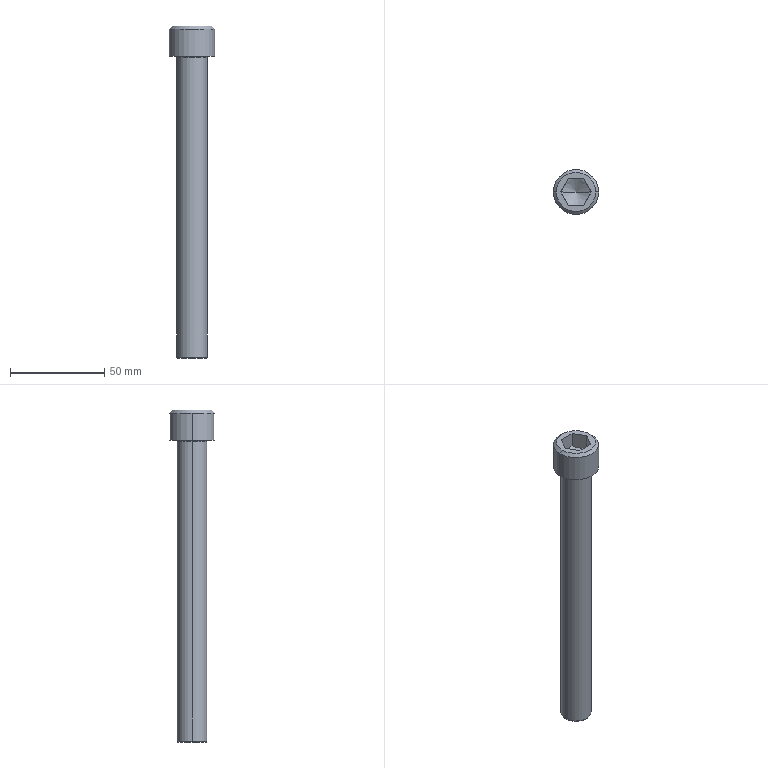Part | Creo | 1 solid | 23 faces | box 24 x 24 x 176 mm | volume 37645 mm3 | plane 9 | cone 6 | cylinder 4 | torus 4 | commonest cylinder face diameters 16 x2 24 x2
STEP:
#1=CARTESIAN_POINT('',(0.,0.,0.));
#2=DIRECTION('',(0.,0.,1.));
#3=DIRECTION('',(1.,0.,0.));
#4=AXIS2_PLACEMENT_3D('',#1,#2,#3);
#5=CARTESIAN_POINT('',(-11.917,-115.,300.5));
#6=VERTEX_POINT('',#5);
#7=CARTESIAN_POINT('',(-15.959,-108.,300.5));
#8=VERTEX_POINT('',#7);
#9=CARTESIAN_POINT('',(-11.917,-115.,300.5));
#10=CARTESIAN_POINT('',(-12.137,-114.619,300.373));
#11=CARTESIAN_POINT('',(-12.578,-113.855,300.149));
#12=CARTESIAN_POINT('',(-13.254,-112.685,299.927));
#13=CARTESIAN_POINT('',(-13.936,-111.504,299.849));
#14=CARTESIAN_POINT('',(-14.621,-110.317,299.927));
#15=CARTESIAN_POINT('',(-15.295,-109.15,300.148));
#16=CARTESIAN_POINT('',(-15.738,-108.382,300.373));
#17=CARTESIAN_POINT('',(-15.959,-108.,300.5));
#18=B_SPLINE_CURVE_WITH_KNOTS('',3,(#9,#10,#11,#12,#13,#14,#15,#16,#17),.UNSPECIFIED.,.F.,.F.,(4,1,1,1,1,1,4),(0.,0.1667,0.3333,0.5,0.6667,0.8333,1.),.UNSPECIFIED.);
#19=EDGE_CURVE('',#6,#8,#18,.T.);
#20=ORIENTED_EDGE('',*,*,#19,.F.);
#21=CARTESIAN_POINT('',(-20.,-115.,295.833));
#22=VERTEX_POINT('',#21);
#23=CARTESIAN_POINT('',(-20.,-115.,295.833));
#24=DIRECTION('',(0.866,0.,0.5));
#25=VECTOR('',#24,9.333);
#26=LINE('',#23,#25);
#27=EDGE_CURVE('',#22,#6,#26,.T.);
#28=ORIENTED_EDGE('',*,*,#27,.F.);
#29=CARTESIAN_POINT('',(-28.083,-115.,300.5));
#30=VERTEX_POINT('',#29);
#31=CARTESIAN_POINT('',(-20.,-115.,295.833));
#32=DIRECTION('',(-0.866,0.,0.5));
#33=VECTOR('',#32,9.333);
#34=LINE('',#31,#33);
#35=EDGE_CURVE('',#22,#30,#34,.T.);
#36=ORIENTED_EDGE('',*,*,#35,.T.);
#37=CARTESIAN_POINT('',(-24.041,-108.,300.5));
#38=VERTEX_POINT('',#37);
#39=CARTESIAN_POINT('',(-24.041,-108.,300.5));
#40=CARTESIAN_POINT('',(-24.261,-108.381,300.373));
#41=CARTESIAN_POINT('',(-24.703,-109.145,300.149));
#42=CARTESIAN_POINT('',(-25.378,-110.315,299.927));
#43=CARTESIAN_POINT('',(-26.06,-111.496,299.849));
#44=CARTESIAN_POINT('',(-26.745,-112.683,299.927));
#45=CARTESIAN_POINT('',(-27.419,-113.85,300.148));
#46=CARTESIAN_POINT('',(-27.862,-114.618,300.373));
#47=CARTESIAN_POINT('',(-28.083,-115.,300.5));
#48=B_SPLINE_CURVE_WITH_KNOTS('',3,(#39,#40,#41,#42,#43,#44,#45,#46,#47),.UNSPECIFIED.,.F.,.F.,(4,1,1,1,1,1,4),(0.,0.1667,0.3333,0.5,0.6667,0.8333,1.),.UNSPECIFIED.);
#49=EDGE_CURVE('',#38,#30,#48,.T.);
#50=ORIENTED_EDGE('',*,*,#49,.F.);
#51=CARTESIAN_POINT('',(-15.959,-108.,300.5));
#52=CARTESIAN_POINT('',(-16.396,-108.,300.374));
#53=CARTESIAN_POINT('',(-17.277,-108.,300.15));
#54=CARTESIAN_POINT('',(-18.631,-108.,299.927));
#55=CARTESIAN_POINT('',(-19.998,-108.,299.849));
#56=CARTESIAN_POINT('',(-21.363,-108.,299.926));
#57=CARTESIAN_POINT('',(-22.717,-108.,300.149));
#58=CARTESIAN_POINT('',(-23.601,-108.,300.373));
#59=CARTESIAN_POINT('',(-24.041,-108.,300.5));
#60=B_SPLINE_CURVE_WITH_KNOTS('',3,(#51,#52,#53,#54,#55,#56,#57,#58,#59),.UNSPECIFIED.,.F.,.F.,(4,1,1,1,1,1,4),(0.,0.1667,0.3333,0.5,0.6667,0.8333,1.),.UNSPECIFIED.);
#61=EDGE_CURVE('',#8,#38,#60,.T.);
#62=ORIENTED_EDGE('',*,*,#61,.F.);
#63=EDGE_LOOP('',(#20,#28,#36,#50,#62));
#64=FACE_OUTER_BOUND('',#63,.F.);
#65=CARTESIAN_POINT('',(-20.,-115.,298.22));
#66=DIRECTION('',(0.,0.,1.));
#67=DIRECTION('',(1.,0.,0.));
#68=AXIS2_PLACEMENT_3D('',#65,#66,#67);
#69=CONICAL_SURFACE('',#68,4.135,60.);
#70=ADVANCED_FACE('',(#64),#69,.F.);
#71=CARTESIAN_POINT('',(-15.959,-108.,308.5));
#72=VERTEX_POINT('',#71);
#73=CARTESIAN_POINT('',(-11.917,-115.,308.5));
#74=VERTEX_POINT('',#73);
#75=CARTESIAN_POINT('',(-15.959,-108.,308.5));
#76=DIRECTION('',(0.5,-0.866,0.));
#77=VECTOR('',#76,8.083);
#78=LINE('',#75,#77);
#79=EDGE_CURVE('',#72,#74,#78,.T.);
#80=ORIENTED_EDGE('',*,*,#79,.T.);
#81=CARTESIAN_POINT('',(-11.917,-115.,308.5));
#82=DIRECTION('',(0.,0.,-1.));
#83=VECTOR('',#82,8.);
#84=LINE('',#81,#83);
#85=EDGE_CURVE('',#74,#6,#84,.T.);
#86=ORIENTED_EDGE('',*,*,#85,.T.);
#87=ORIENTED_EDGE('',*,*,#19,.T.);
#88=CARTESIAN_POINT('',(-15.959,-108.,308.5));
#89=DIRECTION('',(0.,0.,-1.));
#90=VECTOR('',#89,8.);
#91=LINE('',#88,#90);
#92=EDGE_CURVE('',#72,#8,#91,.T.);
#93=ORIENTED_EDGE('',*,*,#92,.F.);
#94=EDGE_LOOP('',(#80,#86,#87,#93));
#95=FACE_OUTER_BOUND('',#94,.F.);
#96=CARTESIAN_POINT('',(-15.959,-108.,300.5));
#97=DIRECTION('',(-0.866,-0.5,0.));
#98=DIRECTION('',(0.5,-0.866,0.));
#99=AXIS2_PLACEMENT_3D('',#96,#97,#98);
#100=PLANE('',#99);
#101=ADVANCED_FACE('',(#95),#100,.T.);
#102=CARTESIAN_POINT('',(-9.6,-115.,308.5));
#103=VERTEX_POINT('',#102);
#104=CARTESIAN_POINT('',(-30.4,-115.,308.5));
#105=VERTEX_POINT('',#104);
#106=CARTESIAN_POINT('',(-20.,-115.,308.5));
#107=DIRECTION('',(0.,0.,1.));
#108=DIRECTION('',(1.,0.,0.));
#109=AXIS2_PLACEMENT_3D('',#106,#107,#108);
#110=CIRCLE('',#109,10.4);
#111=EDGE_CURVE('',#103,#105,#110,.T.);
#112=ORIENTED_EDGE('',*,*,#111,.F.);
#113=CARTESIAN_POINT('',(-20.,-115.,308.5));
#114=DIRECTION('',(0.,0.,1.));
#115=DIRECTION('',(-1.,0.,0.));
#116=AXIS2_PLACEMENT_3D('',#113,#114,#115);
#117=CIRCLE('',#116,10.4);
#118=EDGE_CURVE('',#105,#103,#117,.T.);
#119=ORIENTED_EDGE('',*,*,#118,.F.);
#120=EDGE_LOOP('',(#112,#119));
#121=FACE_OUTER_BOUND('',#120,.F.);
#122=CARTESIAN_POINT('',(-15.959,-122.,308.5));
#123=VERTEX_POINT('',#122);
#124=CARTESIAN_POINT('',(-11.917,-115.,308.5));
#125=DIRECTION('',(-0.5,-0.866,0.));
#126=VECTOR('',#125,8.083);
#127=LINE('',#124,#126);
#128=EDGE_CURVE('',#74,#123,#127,.T.);
#129=ORIENTED_EDGE('',*,*,#128,.F.);
#130=ORIENTED_EDGE('',*,*,#79,.F.);
#131=CARTESIAN_POINT('',(-24.041,-108.,308.5));
#132=VERTEX_POINT('',#131);
#133=CARTESIAN_POINT('',(-15.959,-108.,308.5));
#134=DIRECTION('',(-1.,0.,0.));
#135=VECTOR('',#134,8.083);
#136=LINE('',#133,#135);
#137=EDGE_CURVE('',#72,#132,#136,.T.);
#138=ORIENTED_EDGE('',*,*,#137,.T.);
#139=CARTESIAN_POINT('',(-28.083,-115.,308.5));
#140=VERTEX_POINT('',#139);
#141=CARTESIAN_POINT('',(-28.083,-115.,308.5));
#142=DIRECTION('',(0.5,0.866,0.));
#143=VECTOR('',#142,8.083);
#144=LINE('',#141,#143);
#145=EDGE_CURVE('',#140,#132,#144,.T.);
#146=ORIENTED_EDGE('',*,*,#145,.F.);
#147=CARTESIAN_POINT('',(-24.041,-122.,308.5));
#148=VERTEX_POINT('',#147);
#149=CARTESIAN_POINT('',(-24.041,-122.,308.5));
#150=DIRECTION('',(-0.5,0.866,0.));
#151=VECTOR('',#150,8.083);
#152=LINE('',#149,#151);
#153=EDGE_CURVE('',#148,#140,#152,.T.);
#154=ORIENTED_EDGE('',*,*,#153,.F.);
#155=CARTESIAN_POINT('',(-24.041,-122.,308.5));
#156=DIRECTION('',(1.,0.,0.));
#157=VECTOR('',#156,8.083);
#158=LINE('',#155,#157);
#159=EDGE_CURVE('',#148,#123,#158,.T.);
#160=ORIENTED_EDGE('',*,*,#159,.T.);
#161=EDGE_LOOP('',(#129,#130,#138,#146,#154,#160));
#162=FACE_BOUND('',#161,.F.);
#163=CARTESIAN_POINT('',(-20.,-115.,308.5));
#164=DIRECTION('',(0.,0.,1.));
#165=DIRECTION('',(1.,0.,0.));
#166=AXIS2_PLACEMENT_3D('',#163,#164,#165);
#167=PLANE('',#166);
#168=ADVANCED_FACE('',(#121,#162),#167,.T.);
#169=CARTESIAN_POINT('',(-8.,-115.,306.9));
#170=VERTEX_POINT('',#169);
#171=CARTESIAN_POINT('',(-32.,-115.,306.9));
#172=VERTEX_POINT('',#171);
#173=CARTESIAN_POINT('',(-20.,-115.,306.9));
#174=DIRECTION('',(0.,0.,1.));
#175=DIRECTION('',(1.,0.,0.));
#176=AXIS2_PLACEMENT_3D('',#173,#174,#175);
#177=CIRCLE('',#176,12.);
#178=EDGE_CURVE('',#170,#172,#177,.T.);
#179=ORIENTED_EDGE('',*,*,#178,.F.);
#180=CARTESIAN_POINT('',(-9.6,-115.,308.5));
#181=DIRECTION('',(0.7071,0.,-0.7071));
#182=VECTOR('',#181,2.263);
#183=LINE('',#180,#182);
#184=EDGE_CURVE('',#103,#170,#183,.T.);
#185=ORIENTED_EDGE('',*,*,#184,.F.);
#186=ORIENTED_EDGE('',*,*,#111,.T.);
#187=CARTESIAN_POINT('',(-30.4,-115.,308.5));
#188=DIRECTION('',(-0.7071,0.,-0.7071));
#189=VECTOR('',#188,2.263);
#190=LINE('',#187,#189);
#191=EDGE_CURVE('',#105,#172,#190,.T.);
#192=ORIENTED_EDGE('',*,*,#191,.T.);
#193=EDGE_LOOP('',(#179,#185,#186,#192));
#194=FACE_OUTER_BOUND('',#193,.F.);
#195=CARTESIAN_POINT('',(-20.,-115.,307.7));
#196=DIRECTION('',(0.,0.,-1.));
#197=DIRECTION('',(-1.,0.,0.));
#198=AXIS2_PLACEMENT_3D('',#195,#196,#197);
#199=CONICAL_SURFACE('',#198,11.2,45.);
#200=ADVANCED_FACE('',(#194),#199,.T.);
#201=ORIENTED_EDGE('',*,*,#178,.T.);
#202=CARTESIAN_POINT('',(-32.,-115.,292.5));
#203=VERTEX_POINT('',#202);
#204=CARTESIAN_POINT('',(-32.,-115.,292.5));
#205=DIRECTION('',(0.,0.,1.));
#206=VECTOR('',#205,14.4);
#207=LINE('',#204,#206);
#208=EDGE_CURVE('',#203,#172,#207,.T.);
#209=ORIENTED_EDGE('',*,*,#208,.F.);
#210=CARTESIAN_POINT('',(-8.,-115.,292.5));
#211=VERTEX_POINT('',#210);
#212=CARTESIAN_POINT('',(-20.,-115.,292.5));
#213=DIRECTION('',(0.,0.,-1.));
#214=DIRECTION('',(-1.,0.,0.));
#215=AXIS2_PLACEMENT_3D('',#212,#213,#214);
#216=CIRCLE('',#215,12.);
#217=EDGE_CURVE('',#203,#211,#216,.T.);
#218=ORIENTED_EDGE('',*,*,#217,.T.);
#219=CARTESIAN_POINT('',(-8.,-115.,292.5));
#220=DIRECTION('',(0.,0.,1.));
#221=VECTOR('',#220,14.4);
#222=LINE('',#219,#221);
#223=EDGE_CURVE('',#211,#170,#222,.T.);
#224=ORIENTED_EDGE('',*,*,#223,.T.);
#225=EDGE_LOOP('',(#201,#209,#218,#224));
#226=FACE_OUTER_BOUND('',#225,.F.);
#227=CARTESIAN_POINT('',(-20.,-115.,292.5));
#228=DIRECTION('',(0.,0.,1.));
#229=DIRECTION('',(1.,0.,0.));
#230=AXIS2_PLACEMENT_3D('',#227,#228,#229);
#231=CYLINDRICAL_SURFACE('',#230,12.);
#232=ADVANCED_FACE('',(#226),#231,.T.);
#233=CARTESIAN_POINT('',(-20.,-115.,306.9));
#234=DIRECTION('',(0.,0.,1.));
#235=DIRECTION('',(-1.,0.,0.));
#236=AXIS2_PLACEMENT_3D('',#233,#234,#235);
#237=CIRCLE('',#236,12.);
#238=EDGE_CURVE('',#172,#170,#237,.T.);
#239=ORIENTED_EDGE('',*,*,#238,.T.);
#240=ORIENTED_EDGE('',*,*,#223,.F.);
#241=CARTESIAN_POINT('',(-20.,-115.,292.5));
#242=DIRECTION('',(0.,0.,-1.));
#243=DIRECTION('',(1.,0.,0.));
#244=AXIS2_PLACEMENT_3D('',#241,#242,#243);
#245=CIRCLE('',#244,12.);
#246=EDGE_CURVE('',#211,#203,#245,.T.);
#247=ORIENTED_EDGE('',*,*,#246,.T.);
#248=ORIENTED_EDGE('',*,*,#208,.T.);
#249=EDGE_LOOP('',(#239,#240,#247,#248));
#250=FACE_OUTER_BOUND('',#249,.F.);
#251=CARTESIAN_POINT('',(-20.,-115.,292.5));
#252=DIRECTION('',(0.,0.,1.));
#253=DIRECTION('',(1.,0.,0.));
#254=AXIS2_PLACEMENT_3D('',#251,#252,#253);
#255=CYLINDRICAL_SURFACE('',#254,12.);
#256=ADVANCED_FACE('',(#250),#255,.T.);
#257=ORIENTED_EDGE('',*,*,#238,.F.);
#258=ORIENTED_EDGE('',*,*,#191,.F.);
#259=ORIENTED_EDGE('',*,*,#118,.T.);
#260=ORIENTED_EDGE('',*,*,#184,.T.);
#261=EDGE_LOOP('',(#257,#258,#259,#260));
#262=FACE_OUTER_BOUND('',#261,.F.);
#263=CARTESIAN_POINT('',(-20.,-115.,307.7));
#264=DIRECTION('',(0.,0.,-1.));
#265=DIRECTION('',(-1.,0.,0.));
#266=AXIS2_PLACEMENT_3D('',#263,#264,#265);
#267=CONICAL_SURFACE('',#266,11.2,45.);
#268=ADVANCED_FACE('',(#262),#267,.T.);
#269=ORIENTED_EDGE('',*,*,#246,.F.);
#270=ORIENTED_EDGE('',*,*,#217,.F.);
#271=EDGE_LOOP('',(#269,#270));
#272=FACE_OUTER_BOUND('',#271,.F.);
#273=CARTESIAN_POINT('',(-11.4,-115.,292.5));
#274=VERTEX_POINT('',#273);
#275=CARTESIAN_POINT('',(-28.6,-115.,292.5));
#276=VERTEX_POINT('',#275);
#277=CARTESIAN_POINT('',(-20.,-115.,292.5));
#278=DIRECTION('',(0.,0.,1.));
#279=DIRECTION('',(1.,0.,0.));
#280=AXIS2_PLACEMENT_3D('',#277,#278,#279);
#281=CIRCLE('',#280,8.6);
#282=EDGE_CURVE('',#274,#276,#281,.T.);
#283=ORIENTED_EDGE('',*,*,#282,.F.);
#284=CARTESIAN_POINT('',(-20.,-115.,292.5));
#285=DIRECTION('',(0.,0.,1.));
#286=DIRECTION('',(-1.,0.,0.));
#287=AXIS2_PLACEMENT_3D('',#284,#285,#286);
#288=CIRCLE('',#287,8.6);
#289=EDGE_CURVE('',#276,#274,#288,.T.);
#290=ORIENTED_EDGE('',*,*,#289,.F.);
#291=EDGE_LOOP('',(#283,#290));
#292=FACE_BOUND('',#291,.F.);
#293=CARTESIAN_POINT('',(-20.,-115.,292.5));
#294=DIRECTION('',(0.,0.,1.));
#295=DIRECTION('',(1.,0.,0.));
#296=AXIS2_PLACEMENT_3D('',#293,#294,#295);
#297=PLANE('',#296);
#298=ADVANCED_FACE('',(#272,#292),#297,.F.);
#299=ORIENTED_EDGE('',*,*,#282,.T.);
#300=CARTESIAN_POINT('',(-28.176,-115.,292.324));
#301=VERTEX_POINT('',#300);
#302=CARTESIAN_POINT('',(-28.6,-115.,291.9));
#303=DIRECTION('',(0.,1.,0.));
#304=DIRECTION('',(0.,0.,1.));
#305=AXIS2_PLACEMENT_3D('',#302,#303,#304);
#306=CIRCLE('',#305,0.6);
#307=EDGE_CURVE('',#276,#301,#306,.T.);
#308=ORIENTED_EDGE('',*,*,#307,.T.);
#309=CARTESIAN_POINT('',(-11.824,-115.,292.324));
#310=VERTEX_POINT('',#309);
#311=CARTESIAN_POINT('',(-20.,-115.,292.324));
#312=DIRECTION('',(0.,0.,1.));
#313=DIRECTION('',(1.,0.,0.));
#314=AXIS2_PLACEMENT_3D('',#311,#312,#313);
#315=CIRCLE('',#314,8.176);
#316=EDGE_CURVE('',#310,#301,#315,.T.);
#317=ORIENTED_EDGE('',*,*,#316,.F.);
#318=CARTESIAN_POINT('',(-11.4,-115.,291.9));
#319=DIRECTION('',(0.,-1.,0.));
#320=DIRECTION('',(0.,0.,1.));
#321=AXIS2_PLACEMENT_3D('',#318,#319,#320);
#322=CIRCLE('',#321,0.6);
#323=EDGE_CURVE('',#274,#310,#322,.T.);
#324=ORIENTED_EDGE('',*,*,#323,.F.);
#325=EDGE_LOOP('',(#299,#308,#317,#324));
#326=FACE_OUTER_BOUND('',#325,.F.);
#327=CARTESIAN_POINT('',(-20.,-115.,291.9));
#328=DIRECTION('',(0.,0.,1.));
#329=DIRECTION('',(1.,0.,0.));
#330=AXIS2_PLACEMENT_3D('',#327,#328,#329);
#331=TOROIDAL_SURFACE('',#330,8.6,0.6);
#332=ADVANCED_FACE('',(#326),#331,.F.);
#333=ORIENTED_EDGE('',*,*,#289,.T.);
#334=ORIENTED_EDGE('',*,*,#323,.T.);
#335=CARTESIAN_POINT('',(-20.,-115.,292.324));
#336=DIRECTION('',(0.,0.,1.));
#337=DIRECTION('',(-1.,0.,0.));
#338=AXIS2_PLACEMENT_3D('',#335,#336,#337);
#339=CIRCLE('',#338,8.176);
#340=EDGE_CURVE('',#301,#310,#339,.T.);
#341=ORIENTED_EDGE('',*,*,#340,.F.);
#342=ORIENTED_EDGE('',*,*,#307,.F.);
#343=EDGE_LOOP('',(#333,#334,#341,#342));
#344=FACE_OUTER_BOUND('',#343,.F.);
#345=CARTESIAN_POINT('',(-20.,-115.,291.9));
#346=DIRECTION('',(0.,0.,1.));
#347=DIRECTION('',(1.,0.,0.));
#348=AXIS2_PLACEMENT_3D('',#345,#346,#347);
#349=TOROIDAL_SURFACE('',#348,8.6,0.6);
#350=ADVANCED_FACE('',(#344),#349,.F.);
#351=CARTESIAN_POINT('',(-28.,-115.,291.9));
#352=VERTEX_POINT('',#351);
#353=CARTESIAN_POINT('',(-12.,-115.,291.9));
#354=VERTEX_POINT('',#353);
#355=CARTESIAN_POINT('',(-20.,-115.,291.9));
#356=DIRECTION('',(0.,0.,1.));
#357=DIRECTION('',(-1.,0.,0.));
#358=AXIS2_PLACEMENT_3D('',#355,#356,#357);
#359=CIRCLE('',#358,8.);
#360=EDGE_CURVE('',#352,#354,#359,.T.);
#361=ORIENTED_EDGE('',*,*,#360,.F.);
#362=CARTESIAN_POINT('',(-28.6,-115.,291.9));
#363=DIRECTION('',(0.,1.,0.));
#364=DIRECTION('',(0.7071,0.,0.7071));
#365=AXIS2_PLACEMENT_3D('',#362,#363,#364);
#366=CIRCLE('',#365,0.6);
#367=EDGE_CURVE('',#301,#352,#366,.T.);
#368=ORIENTED_EDGE('',*,*,#367,.F.);
#369=ORIENTED_EDGE('',*,*,#340,.T.);
#370=CARTESIAN_POINT('',(-11.4,-115.,291.9));
#371=DIRECTION('',(0.,-1.,0.));
#372=DIRECTION('',(-0.7071,0.,0.7071));
#373=AXIS2_PLACEMENT_3D('',#370,#371,#372);
#374=CIRCLE('',#373,0.6);
#375=EDGE_CURVE('',#310,#354,#374,.T.);
#376=ORIENTED_EDGE('',*,*,#375,.T.);
#377=EDGE_LOOP('',(#361,#368,#369,#376));
#378=FACE_OUTER_BOUND('',#377,.F.);
#379=CARTESIAN_POINT('',(-20.,-115.,291.9));
#380=DIRECTION('',(0.,0.,1.));
#381=DIRECTION('',(1.,0.,0.));
#382=AXIS2_PLACEMENT_3D('',#379,#380,#381);
#383=TOROIDAL_SURFACE('',#382,8.6,0.6);
#384=ADVANCED_FACE('',(#378),#383,.F.);
#385=CARTESIAN_POINT('',(-12.,-115.,133.));
#386=VERTEX_POINT('',#385);
#387=CARTESIAN_POINT('',(-28.,-115.,133.));
#388=VERTEX_POINT('',#387);
#389=CARTESIAN_POINT('',(-20.,-115.,133.));
#390=DIRECTION('',(0.,0.,-1.));
#391=DIRECTION('',(1.,0.,0.));
#392=AXIS2_PLACEMENT_3D('',#389,#390,#391);
#393=CIRCLE('',#392,8.);
#394=EDGE_CURVE('',#386,#388,#393,.T.);
#395=ORIENTED_EDGE('',*,*,#394,.T.);
#396=CARTESIAN_POINT('',(-28.,-115.,133.));
#397=DIRECTION('',(0.,0.,1.));
#398=VECTOR('',#397,158.9);
#399=LINE('',#396,#398);
#400=EDGE_CURVE('',#388,#352,#399,.T.);
#401=ORIENTED_EDGE('',*,*,#400,.T.);
#402=ORIENTED_EDGE('',*,*,#360,.T.);
#403=CARTESIAN_POINT('',(-12.,-115.,133.));
#404=DIRECTION('',(0.,0.,1.));
#405=VECTOR('',#404,158.9);
#406=LINE('',#403,#405);
#407=EDGE_CURVE('',#386,#354,#406,.T.);
#408=ORIENTED_EDGE('',*,*,#407,.F.);
#409=EDGE_LOOP('',(#395,#401,#402,#408));
#410=FACE_OUTER_BOUND('',#409,.F.);
#411=CARTESIAN_POINT('',(-20.,-115.,132.5));
#412=DIRECTION('',(0.,0.,1.));
#413=DIRECTION('',(1.,0.,0.));
#414=AXIS2_PLACEMENT_3D('',#411,#412,#413);
#415=CYLINDRICAL_SURFACE('',#414,8.);
#416=ADVANCED_FACE('',(#410),#415,.T.);
#417=CARTESIAN_POINT('',(-12.5,-115.,132.5));
#418=VERTEX_POINT('',#417);
#419=CARTESIAN_POINT('',(-27.5,-115.,132.5));
#420=VERTEX_POINT('',#419);
#421=CARTESIAN_POINT('',(-20.,-115.,132.5));
#422=DIRECTION('',(0.,0.,-1.));
#423=DIRECTION('',(1.,0.,0.));
#424=AXIS2_PLACEMENT_3D('',#421,#422,#423);
#425=CIRCLE('',#424,7.5);
#426=EDGE_CURVE('',#418,#420,#425,.T.);
#427=ORIENTED_EDGE('',*,*,#426,.T.);
#428=CARTESIAN_POINT('',(-27.5,-115.,132.5));
#429=DIRECTION('',(-0.7071,0.,0.7071));
#430=VECTOR('',#429,0.7071);
#431=LINE('',#428,#430);
#432=EDGE_CURVE('',#420,#388,#431,.T.);
#433=ORIENTED_EDGE('',*,*,#432,.T.);
#434=ORIENTED_EDGE('',*,*,#394,.F.);
#435=CARTESIAN_POINT('',(-12.5,-115.,132.5));
#436=DIRECTION('',(0.7071,0.,0.7071));
#437=VECTOR('',#436,0.7071);
#438=LINE('',#435,#437);
#439=EDGE_CURVE('',#418,#386,#438,.T.);
#440=ORIENTED_EDGE('',*,*,#439,.F.);
#441=EDGE_LOOP('',(#427,#433,#434,#440));
#442=FACE_OUTER_BOUND('',#441,.F.);
#443=CARTESIAN_POINT('',(-20.,-115.,132.75));
#444=DIRECTION('',(0.,0.,1.));
#445=DIRECTION('',(1.,0.,0.));
#446=AXIS2_PLACEMENT_3D('',#443,#444,#445);
#447=CONICAL_SURFACE('',#446,7.75,45.);
#448=ADVANCED_FACE('',(#442),#447,.T.);
#449=ORIENTED_EDGE('',*,*,#426,.F.);
#450=CARTESIAN_POINT('',(-20.,-115.,132.5));
#451=DIRECTION('',(0.,0.,-1.));
#452=DIRECTION('',(-1.,0.,0.));
#453=AXIS2_PLACEMENT_3D('',#450,#451,#452);
#454=CIRCLE('',#453,7.5);
#455=EDGE_CURVE('',#420,#418,#454,.T.);
#456=ORIENTED_EDGE('',*,*,#455,.F.);
#457=EDGE_LOOP('',(#449,#456));
#458=FACE_OUTER_BOUND('',#457,.F.);
#459=CARTESIAN_POINT('',(-20.,-115.,132.5));
#460=DIRECTION('',(0.,0.,1.));
#461=DIRECTION('',(1.,0.,0.));
#462=AXIS2_PLACEMENT_3D('',#459,#460,#461);
#463=PLANE('',#462);
#464=ADVANCED_FACE('',(#458),#463,.F.);
#465=ORIENTED_EDGE('',*,*,#455,.T.);
#466=ORIENTED_EDGE('',*,*,#439,.T.);
#467=CARTESIAN_POINT('',(-20.,-115.,133.));
#468=DIRECTION('',(0.,0.,-1.));
#469=DIRECTION('',(-1.,0.,0.));
#470=AXIS2_PLACEMENT_3D('',#467,#468,#469);
#471=CIRCLE('',#470,8.);
#472=EDGE_CURVE('',#388,#386,#471,.T.);
#473=ORIENTED_EDGE('',*,*,#472,.F.);
#474=ORIENTED_EDGE('',*,*,#432,.F.);
#475=EDGE_LOOP('',(#465,#466,#473,#474));
#476=FACE_OUTER_BOUND('',#475,.F.);
#477=CARTESIAN_POINT('',(-20.,-115.,132.75));
#478=DIRECTION('',(0.,0.,1.));
#479=DIRECTION('',(1.,0.,0.));
#480=AXIS2_PLACEMENT_3D('',#477,#478,#479);
#481=CONICAL_SURFACE('',#480,7.75,45.);
#482=ADVANCED_FACE('',(#476),#481,.T.);
#483=ORIENTED_EDGE('',*,*,#472,.T.);
#484=ORIENTED_EDGE('',*,*,#407,.T.);
#485=CARTESIAN_POINT('',(-20.,-115.,291.9));
#486=DIRECTION('',(0.,0.,1.));
#487=DIRECTION('',(1.,0.,0.));
#488=AXIS2_PLACEMENT_3D('',#485,#486,#487);
#489=CIRCLE('',#488,8.);
#490=EDGE_CURVE('',#354,#352,#489,.T.);
#491=ORIENTED_EDGE('',*,*,#490,.T.);
#492=ORIENTED_EDGE('',*,*,#400,.F.);
#493=EDGE_LOOP('',(#483,#484,#491,#492));
#494=FACE_OUTER_BOUND('',#493,.F.);
#495=CARTESIAN_POINT('',(-20.,-115.,132.5));
#496=DIRECTION('',(0.,0.,1.));
#497=DIRECTION('',(1.,0.,0.));
#498=AXIS2_PLACEMENT_3D('',#495,#496,#497);
#499=CYLINDRICAL_SURFACE('',#498,8.);
#500=ADVANCED_FACE('',(#494),#499,.T.);
#501=ORIENTED_EDGE('',*,*,#490,.F.);
#502=ORIENTED_EDGE('',*,*,#375,.F.);
#503=ORIENTED_EDGE('',*,*,#316,.T.);
#504=ORIENTED_EDGE('',*,*,#367,.T.);
#505=EDGE_LOOP('',(#501,#502,#503,#504));
#506=FACE_OUTER_BOUND('',#505,.F.);
#507=CARTESIAN_POINT('',(-20.,-115.,291.9));
#508=DIRECTION('',(0.,0.,1.));
#509=DIRECTION('',(1.,0.,0.));
#510=AXIS2_PLACEMENT_3D('',#507,#508,#509);
#511=TOROIDAL_SURFACE('',#510,8.6,0.6);
#512=ADVANCED_FACE('',(#506),#511,.F.);
#513=ORIENTED_EDGE('',*,*,#128,.T.);
#514=CARTESIAN_POINT('',(-15.959,-122.,300.5));
#515=VERTEX_POINT('',#514);
#516=CARTESIAN_POINT('',(-15.959,-122.,308.5));
#517=DIRECTION('',(0.,0.,-1.));
#518=VECTOR('',#517,8.);
#519=LINE('',#516,#518);
#520=EDGE_CURVE('',#123,#515,#519,.T.);
#521=ORIENTED_EDGE('',*,*,#520,.T.);
#522=CARTESIAN_POINT('',(-15.959,-122.,300.5));
#523=CARTESIAN_POINT('',(-15.739,-121.619,300.373));
#524=CARTESIAN_POINT('',(-15.297,-120.855,300.149));
#525=CARTESIAN_POINT('',(-14.622,-119.685,299.927));
#526=CARTESIAN_POINT('',(-13.94,-118.504,299.849));
#527=CARTESIAN_POINT('',(-13.255,-117.317,299.927));
#528=CARTESIAN_POINT('',(-12.581,-116.15,300.148));
#529=CARTESIAN_POINT('',(-12.138,-115.382,300.373));
#530=CARTESIAN_POINT('',(-11.917,-115.,300.5));
#531=B_SPLINE_CURVE_WITH_KNOTS('',3,(#522,#523,#524,#525,#526,#527,#528,#529,#530),.UNSPECIFIED.,.F.,.F.,(4,1,1,1,1,1,4),(0.,0.1667,0.3333,0.5,0.6667,0.8333,1.),.UNSPECIFIED.);
#532=EDGE_CURVE('',#515,#6,#531,.T.);
#533=ORIENTED_EDGE('',*,*,#532,.T.);
#534=ORIENTED_EDGE('',*,*,#85,.F.);
#535=EDGE_LOOP('',(#513,#521,#533,#534));
#536=FACE_OUTER_BOUND('',#535,.F.);
#537=CARTESIAN_POINT('',(-11.917,-115.,300.5));
#538=DIRECTION('',(-0.866,0.5,0.));
#539=DIRECTION('',(-0.5,-0.866,0.));
#540=AXIS2_PLACEMENT_3D('',#537,#538,#539);
#541=PLANE('',#540);
#542=ADVANCED_FACE('',(#536),#541,.T.);
#543=ORIENTED_EDGE('',*,*,#159,.F.);
#544=CARTESIAN_POINT('',(-24.041,-122.,300.5));
#545=VERTEX_POINT('',#544);
#546=CARTESIAN_POINT('',(-24.041,-122.,308.5));
#547=DIRECTION('',(0.,0.,-1.));
#548=VECTOR('',#547,8.);
#549=LINE('',#546,#548);
#550=EDGE_CURVE('',#148,#545,#549,.T.);
#551=ORIENTED_EDGE('',*,*,#550,.T.);
#552=CARTESIAN_POINT('',(-24.041,-122.,300.5));
#553=CARTESIAN_POINT('',(-23.601,-122.,300.373));
#554=CARTESIAN_POINT('',(-22.717,-122.,300.149));
#555=CARTESIAN_POINT('',(-21.363,-122.,299.926));
#556=CARTESIAN_POINT('',(-19.998,-122.,299.849));
#557=CARTESIAN_POINT('',(-18.631,-122.,299.927));
#558=CARTESIAN_POINT('',(-17.277,-122.,300.15));
#559=CARTESIAN_POINT('',(-16.396,-122.,300.374));
#560=CARTESIAN_POINT('',(-15.959,-122.,300.5));
#561=B_SPLINE_CURVE_WITH_KNOTS('',3,(#552,#553,#554,#555,#556,#557,#558,#559,#560),.UNSPECIFIED.,.F.,.F.,(4,1,1,1,1,1,4),(0.,0.1667,0.3333,0.5,0.6667,0.8333,1.),.UNSPECIFIED.);
#562=EDGE_CURVE('',#545,#515,#561,.T.);
#563=ORIENTED_EDGE('',*,*,#562,.T.);
#564=ORIENTED_EDGE('',*,*,#520,.F.);
#565=EDGE_LOOP('',(#543,#551,#563,#564));
#566=FACE_OUTER_BOUND('',#565,.F.);
#567=CARTESIAN_POINT('',(-15.959,-122.,300.5));
#568=DIRECTION('',(0.,1.,0.));
#569=DIRECTION('',(0.,0.,1.));
#570=AXIS2_PLACEMENT_3D('',#567,#568,#569);
#571=PLANE('',#570);
#572=ADVANCED_FACE('',(#566),#571,.T.);
#573=ORIENTED_EDGE('',*,*,#153,.T.);
#574=CARTESIAN_POINT('',(-28.083,-115.,308.5));
#575=DIRECTION('',(0.,0.,-1.));
#576=VECTOR('',#575,8.);
#577=LINE('',#574,#576);
#578=EDGE_CURVE('',#140,#30,#577,.T.);
#579=ORIENTED_EDGE('',*,*,#578,.T.);
#580=CARTESIAN_POINT('',(-28.083,-115.,300.5));
#581=CARTESIAN_POINT('',(-27.862,-115.382,300.373));
#582=CARTESIAN_POINT('',(-27.419,-116.15,300.148));
#583=CARTESIAN_POINT('',(-26.745,-117.317,299.927));
#584=CARTESIAN_POINT('',(-26.06,-118.504,299.849));
#585=CARTESIAN_POINT('',(-25.378,-119.685,299.927));
#586=CARTESIAN_POINT('',(-24.703,-120.855,300.149));
#587=CARTESIAN_POINT('',(-24.261,-121.619,300.373));
#588=CARTESIAN_POINT('',(-24.041,-122.,300.5));
#589=B_SPLINE_CURVE_WITH_KNOTS('',3,(#580,#581,#582,#583,#584,#585,#586,#587,#588),.UNSPECIFIED.,.F.,.F.,(4,1,1,1,1,1,4),(0.,0.1667,0.3333,0.5,0.6667,0.8333,1.),.UNSPECIFIED.);
#590=EDGE_CURVE('',#30,#545,#589,.T.);
#591=ORIENTED_EDGE('',*,*,#590,.T.);
#592=ORIENTED_EDGE('',*,*,#550,.F.);
#593=EDGE_LOOP('',(#573,#579,#591,#592));
#594=FACE_OUTER_BOUND('',#593,.F.);
#595=CARTESIAN_POINT('',(-24.041,-122.,300.5));
#596=DIRECTION('',(0.866,0.5,0.));
#597=DIRECTION('',(-0.5,0.866,0.));
#598=AXIS2_PLACEMENT_3D('',#595,#596,#597);
#599=PLANE('',#598);
#600=ADVANCED_FACE('',(#594),#599,.T.);
#601=ORIENTED_EDGE('',*,*,#145,.T.);
#602=CARTESIAN_POINT('',(-24.041,-108.,308.5));
#603=DIRECTION('',(0.,0.,-1.));
#604=VECTOR('',#603,8.);
#605=LINE('',#602,#604);
#606=EDGE_CURVE('',#132,#38,#605,.T.);
#607=ORIENTED_EDGE('',*,*,#606,.T.);
#608=ORIENTED_EDGE('',*,*,#49,.T.);
#609=ORIENTED_EDGE('',*,*,#578,.F.);
#610=EDGE_LOOP('',(#601,#607,#608,#609));
#611=FACE_OUTER_BOUND('',#610,.F.);
#612=CARTESIAN_POINT('',(-28.083,-115.,300.5));
#613=DIRECTION('',(0.866,-0.5,0.));
#614=DIRECTION('',(0.5,0.866,0.));
#615=AXIS2_PLACEMENT_3D('',#612,#613,#614);
#616=PLANE('',#615);
#617=ADVANCED_FACE('',(#611),#616,.T.);
#618=ORIENTED_EDGE('',*,*,#137,.F.);
#619=ORIENTED_EDGE('',*,*,#92,.T.);
#620=ORIENTED_EDGE('',*,*,#61,.T.);
#621=ORIENTED_EDGE('',*,*,#606,.F.);
#622=EDGE_LOOP('',(#618,#619,#620,#621));
#623=FACE_OUTER_BOUND('',#622,.F.);
#624=CARTESIAN_POINT('',(-24.041,-108.,300.5));
#625=DIRECTION('',(0.,-1.,0.));
#626=DIRECTION('',(0.,0.,-1.));
#627=AXIS2_PLACEMENT_3D('',#624,#625,#626);
#628=PLANE('',#627);
#629=ADVANCED_FACE('',(#623),#628,.T.);
#630=ORIENTED_EDGE('',*,*,#590,.F.);
#631=ORIENTED_EDGE('',*,*,#35,.F.);
#632=ORIENTED_EDGE('',*,*,#27,.T.);
#633=ORIENTED_EDGE('',*,*,#532,.F.);
#634=ORIENTED_EDGE('',*,*,#562,.F.);
#635=EDGE_LOOP('',(#630,#631,#632,#633,#634));
#636=FACE_OUTER_BOUND('',#635,.F.);
#637=CARTESIAN_POINT('',(-20.,-115.,298.22));
#638=DIRECTION('',(0.,0.,1.));
#639=DIRECTION('',(1.,0.,0.));
#640=AXIS2_PLACEMENT_3D('',#637,#638,#639);
#641=CONICAL_SURFACE('',#640,4.135,60.);
#642=ADVANCED_FACE('',(#636),#641,.F.);
#643=CLOSED_SHELL('',(#70,#101,#168,#200,#232,#256,#268,#298,#332,#350,#384,#416,#448,#464,#482,#500,#512,#542,#572,#600,#617,#629,#642));
#644=MANIFOLD_SOLID_BREP('',#643);
#645=(LENGTH_UNIT()NAMED_UNIT(*)SI_UNIT(.MILLI.,.METRE.));
#646=UNCERTAINTY_MEASURE_WITH_UNIT(LENGTH_MEASURE(0.01792),#645,'','');
#647=(NAMED_UNIT(*)PLANE_ANGLE_UNIT()SI_UNIT($,.RADIAN.));
#648=PLANE_ANGLE_MEASURE_WITH_UNIT(PLANE_ANGLE_MEASURE(0.01745),#647);
#649=(CONVERSION_BASED_UNIT('DEGREE',#648)NAMED_UNIT(*)PLANE_ANGLE_UNIT());
#650=(NAMED_UNIT(*)SI_UNIT($,.STERADIAN.)SOLID_ANGLE_UNIT());
#651=(GEOMETRIC_REPRESENTATION_CONTEXT(3)GLOBAL_UNCERTAINTY_ASSIGNED_CONTEXT((#646))GLOBAL_UNIT_ASSIGNED_CONTEXT((#645,#649,#650))REPRESENTATION_CONTEXT('',''));
#652=ADVANCED_BREP_SHAPE_REPRESENTATION('',(#4,#644),#651);